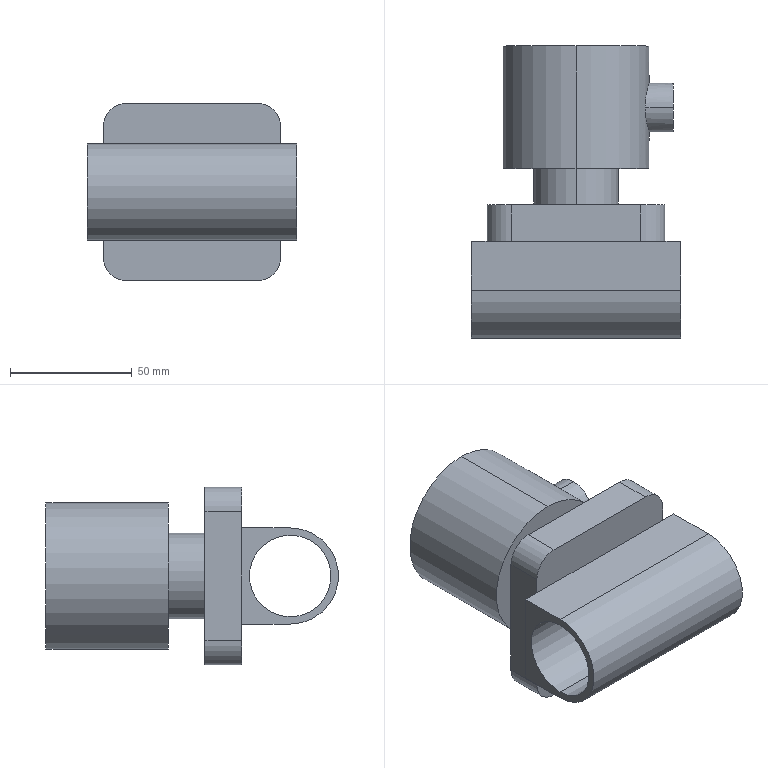Part | SolidWorks | features ICE 5, ExtruThin 1 | 1 solid | 29 faces | box 86 x 120 x 73 mm | volume 283263 mm3 | plane 16 | cylinder 13 | commonest cylinder face diameters 20 x6 33.5 x2 35 x2 60 x2 39.5 x1
STEP:
#1=CARTESIAN_POINT('',(28.284,75.,-10.));
#2=VERTEX_POINT('',#1);
#3=CARTESIAN_POINT('',(28.284,75.,10.));
#4=VERTEX_POINT('',#3);
#5=CARTESIAN_POINT('',(28.284,75.,-10.));
#6=CARTESIAN_POINT('',(28.284,75.666,-10.));
#7=CARTESIAN_POINT('',(28.308,76.32,-9.934));
#8=CARTESIAN_POINT('',(28.374,77.283,-9.741));
#9=CARTESIAN_POINT('',(28.402,77.601,-9.661));
#10=CARTESIAN_POINT('',(28.467,78.232,-9.469));
#11=CARTESIAN_POINT('',(28.504,78.544,-9.357));
#12=CARTESIAN_POINT('',(28.626,79.45,-8.979));
#13=CARTESIAN_POINT('',(28.722,80.023,-8.672));
#14=CARTESIAN_POINT('',(28.879,80.835,-8.128));
#15=CARTESIAN_POINT('',(28.933,81.099,-7.931));
#16=CARTESIAN_POINT('',(29.044,81.603,-7.517));
#17=CARTESIAN_POINT('',(29.1,81.844,-7.299));
#18=CARTESIAN_POINT('',(29.266,82.53,-6.612));
#19=CARTESIAN_POINT('',(29.376,82.942,-6.112));
#20=CARTESIAN_POINT('',(29.582,83.674,-5.02));
#21=CARTESIAN_POINT('',(29.675,83.981,-4.445));
#22=CARTESIAN_POINT('',(29.791,84.357,-3.544));
#23=CARTESIAN_POINT('',(29.827,84.467,-3.237));
#24=CARTESIAN_POINT('',(29.888,84.66,-2.608));
#25=CARTESIAN_POINT('',(29.915,84.741,-2.285));
#26=CARTESIAN_POINT('',(29.978,84.935,-1.315));
#27=CARTESIAN_POINT('',(30.,85.,-0.6623));
#28=CARTESIAN_POINT('',(30.,85.,0.3243));
#29=CARTESIAN_POINT('',(29.995,84.984,0.6555));
#30=CARTESIAN_POINT('',(29.973,84.918,1.317));
#31=CARTESIAN_POINT('',(29.957,84.87,1.643));
#32=CARTESIAN_POINT('',(29.893,84.676,2.608));
#33=CARTESIAN_POINT('',(29.831,84.486,3.234));
#34=CARTESIAN_POINT('',(29.714,84.106,4.147));
#35=CARTESIAN_POINT('',(29.67,83.964,4.445));
#36=CARTESIAN_POINT('',(29.579,83.655,5.02));
#37=CARTESIAN_POINT('',(29.53,83.487,5.298));
#38=CARTESIAN_POINT('',(29.428,83.126,5.837));
#39=CARTESIAN_POINT('',(29.375,82.932,6.098));
#40=CARTESIAN_POINT('',(29.266,82.518,6.602));
#41=CARTESIAN_POINT('',(29.209,82.297,6.846));
#42=CARTESIAN_POINT('',(29.042,81.606,7.536));
#43=CARTESIAN_POINT('',(28.931,81.106,7.946));
#44=CARTESIAN_POINT('',(28.722,80.026,8.67));
#45=CARTESIAN_POINT('',(28.625,79.441,8.984));
#46=CARTESIAN_POINT('',(28.463,78.237,9.484));
#47=CARTESIAN_POINT('',(28.397,77.613,9.675));
#48=CARTESIAN_POINT('',(28.33,76.643,9.87));
#49=CARTESIAN_POINT('',(28.313,76.312,9.919));
#50=CARTESIAN_POINT('',(28.29,75.656,9.984));
#51=CARTESIAN_POINT('',(28.284,75.328,10.));
#52=CARTESIAN_POINT('',(28.284,75.,10.));
#53=B_SPLINE_CURVE_WITH_KNOTS('',3,(#5,#6,#7,#8,#9,#10,#11,#12,#13,#14,#15,#16,#17,#18,#19,#20,#21,#22,#23,#24,#25,#26,#27,#28,#29,#30,#31,#32,#33,#34,#35,#36,#37,#38,#39,#40,#41,#42,#43,#44,#45,#46,#47,#48,#49,#50,#51,#52),.UNSPECIFIED.,.F.,.F.,(4,2,2,2,2,2,2,2,2,2,2,2,2,2,2,2,2,2,2,2,2,2,2,4),(0.,0.001968,0.002952,0.003936,0.005905,0.006889,0.007873,0.009841,0.01181,0.01279,0.01378,0.01575,0.01673,0.01771,0.01968,0.02067,0.02165,0.02263,0.02362,0.02559,0.02755,0.02952,0.03051,0.03149),.UNSPECIFIED.);
#54=EDGE_CURVE('',#2,#4,#53,.T.);
#55=ORIENTED_EDGE('',*,*,#54,.T.);
#56=CARTESIAN_POINT('',(40.,75.,10.));
#57=VERTEX_POINT('',#56);
#58=CARTESIAN_POINT('',(-43.001,75.,10.));
#59=DIRECTION('',(1.,0.,0.));
#60=VECTOR('',#59,1000.);
#61=LINE('',#58,#60);
#62=EDGE_CURVE('',#4,#57,#61,.T.);
#63=ORIENTED_EDGE('',*,*,#62,.T.);
#64=CARTESIAN_POINT('',(40.,75.,-10.));
#65=VERTEX_POINT('',#64);
#66=CARTESIAN_POINT('',(40.,75.,0.));
#67=DIRECTION('',(1.,0.,0.));
#68=DIRECTION('',(0.,0.,-1.));
#69=AXIS2_PLACEMENT_3D('',#66,#67,#68);
#70=CIRCLE('',#69,10.);
#71=EDGE_CURVE('',#65,#57,#70,.T.);
#72=ORIENTED_EDGE('',*,*,#71,.F.);
#73=CARTESIAN_POINT('',(-43.001,75.,-10.));
#74=DIRECTION('',(1.,0.,0.));
#75=VECTOR('',#74,1000.);
#76=LINE('',#73,#75);
#77=EDGE_CURVE('',#2,#65,#76,.T.);
#78=ORIENTED_EDGE('',*,*,#77,.F.);
#79=EDGE_LOOP('',(#55,#63,#72,#78));
#80=FACE_OUTER_BOUND('',#79,.T.);
#81=CARTESIAN_POINT('',(-43.001,75.,0.));
#82=DIRECTION('',(1.,0.,0.));
#83=DIRECTION('',(0.,0.,-1.));
#84=AXIS2_PLACEMENT_3D('',#81,#82,#83);
#85=CYLINDRICAL_SURFACE('',#84,10.);
#86=ADVANCED_FACE('',(#80),#85,.T.);
#87=ORIENTED_EDGE('',*,*,#54,.F.);
#88=CARTESIAN_POINT('',(28.284,75.,10.));
#89=CARTESIAN_POINT('',(28.284,74.672,10.));
#90=CARTESIAN_POINT('',(28.29,74.344,9.984));
#91=CARTESIAN_POINT('',(28.313,73.689,9.919));
#92=CARTESIAN_POINT('',(28.33,73.36,9.87));
#93=CARTESIAN_POINT('',(28.397,72.387,9.675));
#94=CARTESIAN_POINT('',(28.463,71.762,9.484));
#95=CARTESIAN_POINT('',(28.625,70.556,8.982));
#96=CARTESIAN_POINT('',(28.723,69.971,8.668));
#97=CARTESIAN_POINT('',(28.931,68.892,7.944));
#98=CARTESIAN_POINT('',(29.043,68.391,7.533));
#99=CARTESIAN_POINT('',(29.211,67.699,6.841));
#100=CARTESIAN_POINT('',(29.267,67.478,6.597));
#101=CARTESIAN_POINT('',(29.375,67.065,6.095));
#102=CARTESIAN_POINT('',(29.428,66.872,5.835));
#103=CARTESIAN_POINT('',(29.53,66.512,5.296));
#104=CARTESIAN_POINT('',(29.579,66.344,5.018));
#105=CARTESIAN_POINT('',(29.671,66.036,4.444));
#106=CARTESIAN_POINT('',(29.714,65.894,4.145));
#107=CARTESIAN_POINT('',(29.832,65.514,3.233));
#108=CARTESIAN_POINT('',(29.893,65.324,2.609));
#109=CARTESIAN_POINT('',(29.957,65.131,1.646));
#110=CARTESIAN_POINT('',(29.973,65.082,1.32));
#111=CARTESIAN_POINT('',(29.995,65.016,0.6609));
#112=CARTESIAN_POINT('',(30.,65.,0.328));
#113=CARTESIAN_POINT('',(30.,65.,-0.6604));
#114=CARTESIAN_POINT('',(29.978,65.065,-1.313));
#115=CARTESIAN_POINT('',(29.915,65.258,-2.282));
#116=CARTESIAN_POINT('',(29.888,65.34,-2.606));
#117=CARTESIAN_POINT('',(29.827,65.532,-3.235));
#118=CARTESIAN_POINT('',(29.792,65.643,-3.543));
#119=CARTESIAN_POINT('',(29.714,65.894,-4.145));
#120=CARTESIAN_POINT('',(29.671,66.034,-4.44));
#121=CARTESIAN_POINT('',(29.579,66.342,-5.015));
#122=CARTESIAN_POINT('',(29.53,66.512,-5.297));
#123=CARTESIAN_POINT('',(29.376,67.059,-6.113));
#124=CARTESIAN_POINT('',(29.266,67.471,-6.614));
#125=CARTESIAN_POINT('',(29.099,68.159,-7.301));
#126=CARTESIAN_POINT('',(29.043,68.4,-7.519));
#127=CARTESIAN_POINT('',(28.932,68.905,-7.935));
#128=CARTESIAN_POINT('',(28.878,69.169,-8.13));
#129=CARTESIAN_POINT('',(28.722,69.979,-8.672));
#130=CARTESIAN_POINT('',(28.626,70.55,-8.979));
#131=CARTESIAN_POINT('',(28.504,71.457,-9.357));
#132=CARTESIAN_POINT('',(28.467,71.769,-9.469));
#133=CARTESIAN_POINT('',(28.402,72.399,-9.661));
#134=CARTESIAN_POINT('',(28.374,72.717,-9.741));
#135=CARTESIAN_POINT('',(28.308,73.68,-9.934));
#136=CARTESIAN_POINT('',(28.284,74.334,-10.));
#137=CARTESIAN_POINT('',(28.284,75.,-10.));
#138=B_SPLINE_CURVE_WITH_KNOTS('',3,(#88,#89,#90,#91,#92,#93,#94,#95,#96,#97,#98,#99,#100,#101,#102,#103,#104,#105,#106,#107,#108,#109,#110,#111,#112,#113,#114,#115,#116,#117,#118,#119,#120,#121,#122,#123,#124,#125,#126,#127,#128,#129,#130,#131,#132,#133,#134,#135,#136,#137),.UNSPECIFIED.,.F.,.F.,(4,2,2,2,2,2,2,2,2,2,2,2,2,2,2,2,2,2,2,2,2,2,2,2,4),(0.03149,0.03247,0.03346,0.03543,0.03739,0.03936,0.04035,0.04133,0.04231,0.0433,0.04526,0.04625,0.04723,0.0492,0.05018,0.05117,0.05215,0.05313,0.0551,0.05609,0.05707,0.05904,0.06002,0.06101,0.06297),.UNSPECIFIED.);
#139=EDGE_CURVE('',#4,#2,#138,.T.);
#140=ORIENTED_EDGE('',*,*,#139,.F.);
#141=EDGE_LOOP('',(#87,#140));
#142=FACE_BOUND('',#141,.T.);
#143=CARTESIAN_POINT('',(0.,100.25,30.));
#144=VERTEX_POINT('',#143);
#145=CARTESIAN_POINT('',(0.,100.25,-30.));
#146=VERTEX_POINT('',#145);
#147=CARTESIAN_POINT('',(0.,100.25,0.));
#148=DIRECTION('',(0.,1.,0.));
#149=DIRECTION('',(0.,0.,1.));
#150=AXIS2_PLACEMENT_3D('',#147,#148,#149);
#151=CIRCLE('',#150,30.);
#152=EDGE_CURVE('',#144,#146,#151,.T.);
#153=ORIENTED_EDGE('',*,*,#152,.F.);
#154=CARTESIAN_POINT('',(0.,50.,30.));
#155=VERTEX_POINT('',#154);
#156=CARTESIAN_POINT('',(0.,100.25,30.));
#157=DIRECTION('',(0.,-1.,0.));
#158=VECTOR('',#157,1000.);
#159=LINE('',#156,#158);
#160=EDGE_CURVE('',#144,#155,#159,.T.);
#161=ORIENTED_EDGE('',*,*,#160,.T.);
#162=CARTESIAN_POINT('',(0.,50.,-30.));
#163=VERTEX_POINT('',#162);
#164=CARTESIAN_POINT('',(0.,50.,0.));
#165=DIRECTION('',(0.,1.,0.));
#166=DIRECTION('',(0.,0.,1.));
#167=AXIS2_PLACEMENT_3D('',#164,#165,#166);
#168=CIRCLE('',#167,30.);
#169=EDGE_CURVE('',#155,#163,#168,.T.);
#170=ORIENTED_EDGE('',*,*,#169,.T.);
#171=CARTESIAN_POINT('',(0.,100.25,-30.));
#172=DIRECTION('',(0.,-1.,0.));
#173=VECTOR('',#172,1000.);
#174=LINE('',#171,#173);
#175=EDGE_CURVE('',#146,#163,#174,.T.);
#176=ORIENTED_EDGE('',*,*,#175,.F.);
#177=EDGE_LOOP('',(#153,#161,#170,#176));
#178=FACE_OUTER_BOUND('',#177,.T.);
#179=CARTESIAN_POINT('',(0.,100.25,0.));
#180=DIRECTION('',(0.,-1.,0.));
#181=DIRECTION('',(0.,0.,-1.));
#182=AXIS2_PLACEMENT_3D('',#179,#180,#181);
#183=CYLINDRICAL_SURFACE('',#182,30.);
#184=ADVANCED_FACE('',(#142,#178),#183,.T.);
#185=CARTESIAN_POINT('',(0.,50.,17.5));
#186=VERTEX_POINT('',#185);
#187=CARTESIAN_POINT('',(0.,50.,-17.5));
#188=VERTEX_POINT('',#187);
#189=CARTESIAN_POINT('',(0.,50.,0.));
#190=DIRECTION('',(0.,1.,0.));
#191=DIRECTION('',(0.,0.,1.));
#192=AXIS2_PLACEMENT_3D('',#189,#190,#191);
#193=CIRCLE('',#192,17.5);
#194=EDGE_CURVE('',#186,#188,#193,.T.);
#195=ORIENTED_EDGE('',*,*,#194,.F.);
#196=CARTESIAN_POINT('',(0.,35.,17.5));
#197=VERTEX_POINT('',#196);
#198=CARTESIAN_POINT('',(0.,50.,17.5));
#199=DIRECTION('',(0.,-1.,0.));
#200=VECTOR('',#199,1000.);
#201=LINE('',#198,#200);
#202=EDGE_CURVE('',#186,#197,#201,.T.);
#203=ORIENTED_EDGE('',*,*,#202,.T.);
#204=CARTESIAN_POINT('',(0.,35.,-17.5));
#205=VERTEX_POINT('',#204);
#206=CARTESIAN_POINT('',(0.,35.,0.));
#207=DIRECTION('',(0.,1.,0.));
#208=DIRECTION('',(0.,0.,-1.));
#209=AXIS2_PLACEMENT_3D('',#206,#207,#208);
#210=CIRCLE('',#209,17.5);
#211=EDGE_CURVE('',#197,#205,#210,.T.);
#212=ORIENTED_EDGE('',*,*,#211,.T.);
#213=CARTESIAN_POINT('',(0.,50.,-17.5));
#214=DIRECTION('',(0.,-1.,0.));
#215=VECTOR('',#214,1000.);
#216=LINE('',#213,#215);
#217=EDGE_CURVE('',#188,#205,#216,.T.);
#218=ORIENTED_EDGE('',*,*,#217,.F.);
#219=EDGE_LOOP('',(#195,#203,#212,#218));
#220=FACE_OUTER_BOUND('',#219,.T.);
#221=CARTESIAN_POINT('',(0.,50.,0.));
#222=DIRECTION('',(0.,-1.,0.));
#223=DIRECTION('',(0.,0.,-1.));
#224=AXIS2_PLACEMENT_3D('',#221,#222,#223);
#225=CYLINDRICAL_SURFACE('',#224,17.5);
#226=ADVANCED_FACE('',(#220),#225,.T.);
#227=CARTESIAN_POINT('',(43.,0.,16.75));
#228=VERTEX_POINT('',#227);
#229=CARTESIAN_POINT('',(43.,0.,-16.75));
#230=VERTEX_POINT('',#229);
#231=CARTESIAN_POINT('',(43.,0.,0.));
#232=DIRECTION('',(1.,0.,0.));
#233=DIRECTION('',(0.,0.,-1.));
#234=AXIS2_PLACEMENT_3D('',#231,#232,#233);
#235=CIRCLE('',#234,16.75);
#236=EDGE_CURVE('',#228,#230,#235,.T.);
#237=ORIENTED_EDGE('',*,*,#236,.T.);
#238=CARTESIAN_POINT('',(-43.,0.,-16.75));
#239=VERTEX_POINT('',#238);
#240=CARTESIAN_POINT('',(43.,0.,-16.75));
#241=DIRECTION('',(-1.,0.,0.));
#242=VECTOR('',#241,1000.);
#243=LINE('',#240,#242);
#244=EDGE_CURVE('',#230,#239,#243,.T.);
#245=ORIENTED_EDGE('',*,*,#244,.T.);
#246=CARTESIAN_POINT('',(-43.,0.,16.75));
#247=VERTEX_POINT('',#246);
#248=CARTESIAN_POINT('',(-43.,0.,0.));
#249=DIRECTION('',(1.,0.,0.));
#250=DIRECTION('',(0.,0.,-1.));
#251=AXIS2_PLACEMENT_3D('',#248,#249,#250);
#252=CIRCLE('',#251,16.75);
#253=EDGE_CURVE('',#247,#239,#252,.T.);
#254=ORIENTED_EDGE('',*,*,#253,.F.);
#255=CARTESIAN_POINT('',(43.,0.,16.75));
#256=DIRECTION('',(-1.,0.,0.));
#257=VECTOR('',#256,1000.);
#258=LINE('',#255,#257);
#259=EDGE_CURVE('',#228,#247,#258,.T.);
#260=ORIENTED_EDGE('',*,*,#259,.F.);
#261=EDGE_LOOP('',(#237,#245,#254,#260));
#262=FACE_OUTER_BOUND('',#261,.T.);
#263=CARTESIAN_POINT('',(43.,0.,0.));
#264=DIRECTION('',(-1.,0.,0.));
#265=DIRECTION('',(0.,0.,1.));
#266=AXIS2_PLACEMENT_3D('',#263,#264,#265);
#267=CYLINDRICAL_SURFACE('',#266,16.75);
#268=ADVANCED_FACE('',(#262),#267,.F.);
#269=CARTESIAN_POINT('',(-36.5,20.,-19.75));
#270=VERTEX_POINT('',#269);
#271=CARTESIAN_POINT('',(-36.5,20.,19.75));
#272=VERTEX_POINT('',#271);
#273=CARTESIAN_POINT('',(-36.5,20.,-26.5));
#274=DIRECTION('',(0.,0.,1.));
#275=VECTOR('',#274,1000.);
#276=LINE('',#273,#275);
#277=EDGE_CURVE('',#270,#272,#276,.T.);
#278=ORIENTED_EDGE('',*,*,#277,.F.);
#279=CARTESIAN_POINT('',(-43.,20.,-19.75));
#280=VERTEX_POINT('',#279);
#281=CARTESIAN_POINT('',(-87.275,20.,-19.75));
#282=DIRECTION('',(1.,0.,0.));
#283=VECTOR('',#282,1000.);
#284=LINE('',#281,#283);
#285=EDGE_CURVE('',#280,#270,#284,.T.);
#286=ORIENTED_EDGE('',*,*,#285,.F.);
#287=CARTESIAN_POINT('',(-43.,20.,19.75));
#288=VERTEX_POINT('',#287);
#289=CARTESIAN_POINT('',(-43.,20.,19.75));
#290=DIRECTION('',(0.,0.,-1.));
#291=VECTOR('',#290,1000.);
#292=LINE('',#289,#291);
#293=EDGE_CURVE('',#288,#280,#292,.T.);
#294=ORIENTED_EDGE('',*,*,#293,.F.);
#295=CARTESIAN_POINT('',(-87.275,20.,19.75));
#296=DIRECTION('',(1.,0.,0.));
#297=VECTOR('',#296,1000.);
#298=LINE('',#295,#297);
#299=EDGE_CURVE('',#288,#272,#298,.T.);
#300=ORIENTED_EDGE('',*,*,#299,.T.);
#301=EDGE_LOOP('',(#278,#286,#294,#300));
#302=FACE_OUTER_BOUND('',#301,.T.);
#303=CARTESIAN_POINT('',(-87.275,20.,19.75));
#304=DIRECTION('',(0.,1.,0.));
#305=DIRECTION('',(0.,0.,1.));
#306=AXIS2_PLACEMENT_3D('',#303,#304,#305);
#307=PLANE('',#306);
#308=ADVANCED_FACE('',(#302),#307,.T.);
#309=CARTESIAN_POINT('',(43.,0.,19.75));
#310=VERTEX_POINT('',#309);
#311=CARTESIAN_POINT('',(43.,0.,-19.75));
#312=VERTEX_POINT('',#311);
#313=CARTESIAN_POINT('',(43.,0.,0.));
#314=DIRECTION('',(1.,0.,0.));
#315=DIRECTION('',(0.,0.,-1.));
#316=AXIS2_PLACEMENT_3D('',#313,#314,#315);
#317=CIRCLE('',#316,19.75);
#318=EDGE_CURVE('',#310,#312,#317,.T.);
#319=ORIENTED_EDGE('',*,*,#318,.T.);
#320=CARTESIAN_POINT('',(43.,20.,-19.75));
#321=VERTEX_POINT('',#320);
#322=CARTESIAN_POINT('',(43.,0.,-19.75));
#323=DIRECTION('',(0.,1.,0.));
#324=VECTOR('',#323,1000.);
#325=LINE('',#322,#324);
#326=EDGE_CURVE('',#312,#321,#325,.T.);
#327=ORIENTED_EDGE('',*,*,#326,.T.);
#328=CARTESIAN_POINT('',(43.,20.,19.75));
#329=VERTEX_POINT('',#328);
#330=CARTESIAN_POINT('',(43.,20.,19.75));
#331=DIRECTION('',(0.,0.,1.));
#332=VECTOR('',#331,1000.);
#333=LINE('',#330,#332);
#334=EDGE_CURVE('',#321,#329,#333,.T.);
#335=ORIENTED_EDGE('',*,*,#334,.T.);
#336=CARTESIAN_POINT('',(43.,0.,19.75));
#337=DIRECTION('',(0.,-1.,0.));
#338=VECTOR('',#337,1000.);
#339=LINE('',#336,#338);
#340=EDGE_CURVE('',#329,#310,#339,.T.);
#341=ORIENTED_EDGE('',*,*,#340,.T.);
#342=EDGE_LOOP('',(#319,#327,#335,#341));
#343=FACE_OUTER_BOUND('',#342,.T.);
#344=ORIENTED_EDGE('',*,*,#236,.F.);
#345=CARTESIAN_POINT('',(43.,0.,0.));
#346=DIRECTION('',(1.,0.,0.));
#347=DIRECTION('',(0.,0.,-1.));
#348=AXIS2_PLACEMENT_3D('',#345,#346,#347);
#349=CIRCLE('',#348,16.75);
#350=EDGE_CURVE('',#230,#228,#349,.T.);
#351=ORIENTED_EDGE('',*,*,#350,.F.);
#352=EDGE_LOOP('',(#344,#351));
#353=FACE_BOUND('',#352,.T.);
#354=CARTESIAN_POINT('',(43.,0.,0.));
#355=DIRECTION('',(1.,0.,0.));
#356=DIRECTION('',(0.,0.,-1.));
#357=AXIS2_PLACEMENT_3D('',#354,#355,#356);
#358=PLANE('',#357);
#359=ADVANCED_FACE('',(#343,#353),#358,.T.);
#360=CARTESIAN_POINT('',(-43.,0.,19.75));
#361=VERTEX_POINT('',#360);
#362=CARTESIAN_POINT('',(-43.,0.,-19.75));
#363=VERTEX_POINT('',#362);
#364=CARTESIAN_POINT('',(-43.,0.,0.));
#365=DIRECTION('',(1.,0.,0.));
#366=DIRECTION('',(0.,0.,-1.));
#367=AXIS2_PLACEMENT_3D('',#364,#365,#366);
#368=CIRCLE('',#367,19.75);
#369=EDGE_CURVE('',#361,#363,#368,.T.);
#370=ORIENTED_EDGE('',*,*,#369,.F.);
#371=CARTESIAN_POINT('',(-43.,0.,19.75));
#372=DIRECTION('',(0.,1.,0.));
#373=VECTOR('',#372,1000.);
#374=LINE('',#371,#373);
#375=EDGE_CURVE('',#361,#288,#374,.T.);
#376=ORIENTED_EDGE('',*,*,#375,.T.);
#377=ORIENTED_EDGE('',*,*,#293,.T.);
#378=CARTESIAN_POINT('',(-43.,0.,-19.75));
#379=DIRECTION('',(0.,-1.,0.));
#380=VECTOR('',#379,1000.);
#381=LINE('',#378,#380);
#382=EDGE_CURVE('',#280,#363,#381,.T.);
#383=ORIENTED_EDGE('',*,*,#382,.T.);
#384=EDGE_LOOP('',(#370,#376,#377,#383));
#385=FACE_OUTER_BOUND('',#384,.T.);
#386=ORIENTED_EDGE('',*,*,#253,.T.);
#387=CARTESIAN_POINT('',(-43.,0.,0.));
#388=DIRECTION('',(1.,0.,0.));
#389=DIRECTION('',(0.,0.,-1.));
#390=AXIS2_PLACEMENT_3D('',#387,#388,#389);
#391=CIRCLE('',#390,16.75);
#392=EDGE_CURVE('',#239,#247,#391,.T.);
#393=ORIENTED_EDGE('',*,*,#392,.T.);
#394=EDGE_LOOP('',(#386,#393));
#395=FACE_BOUND('',#394,.T.);
#396=CARTESIAN_POINT('',(-43.,0.,0.));
#397=DIRECTION('',(1.,0.,0.));
#398=DIRECTION('',(0.,0.,-1.));
#399=AXIS2_PLACEMENT_3D('',#396,#397,#398);
#400=PLANE('',#399);
#401=ADVANCED_FACE('',(#385,#395),#400,.F.);
#402=ORIENTED_EDGE('',*,*,#318,.F.);
#403=CARTESIAN_POINT('',(-87.275,0.,19.75));
#404=DIRECTION('',(1.,0.,0.));
#405=VECTOR('',#404,1000.);
#406=LINE('',#403,#405);
#407=EDGE_CURVE('',#361,#310,#406,.T.);
#408=ORIENTED_EDGE('',*,*,#407,.F.);
#409=ORIENTED_EDGE('',*,*,#369,.T.);
#410=CARTESIAN_POINT('',(-87.275,0.,-19.75));
#411=DIRECTION('',(1.,0.,0.));
#412=VECTOR('',#411,1000.);
#413=LINE('',#410,#412);
#414=EDGE_CURVE('',#363,#312,#413,.T.);
#415=ORIENTED_EDGE('',*,*,#414,.T.);
#416=EDGE_LOOP('',(#402,#408,#409,#415));
#417=FACE_OUTER_BOUND('',#416,.T.);
#418=CARTESIAN_POINT('',(43.,0.,0.));
#419=DIRECTION('',(-1.,0.,0.));
#420=DIRECTION('',(0.,0.,1.));
#421=AXIS2_PLACEMENT_3D('',#418,#419,#420);
#422=CYLINDRICAL_SURFACE('',#421,19.75);
#423=ADVANCED_FACE('',(#417),#422,.T.);
#424=ORIENTED_EDGE('',*,*,#244,.F.);
#425=ORIENTED_EDGE('',*,*,#350,.T.);
#426=ORIENTED_EDGE('',*,*,#259,.T.);
#427=ORIENTED_EDGE('',*,*,#392,.F.);
#428=EDGE_LOOP('',(#424,#425,#426,#427));
#429=FACE_OUTER_BOUND('',#428,.T.);
#430=CARTESIAN_POINT('',(43.,0.,0.));
#431=DIRECTION('',(-1.,0.,0.));
#432=DIRECTION('',(0.,0.,1.));
#433=AXIS2_PLACEMENT_3D('',#430,#431,#432);
#434=CYLINDRICAL_SURFACE('',#433,16.75);
#435=ADVANCED_FACE('',(#429),#434,.F.);
#436=ORIENTED_EDGE('',*,*,#375,.F.);
#437=ORIENTED_EDGE('',*,*,#407,.T.);
#438=ORIENTED_EDGE('',*,*,#340,.F.);
#439=CARTESIAN_POINT('',(36.5,20.,19.75));
#440=VERTEX_POINT('',#439);
#441=CARTESIAN_POINT('',(-87.275,20.,19.75));
#442=DIRECTION('',(1.,0.,0.));
#443=VECTOR('',#442,1000.);
#444=LINE('',#441,#443);
#445=EDGE_CURVE('',#440,#329,#444,.T.);
#446=ORIENTED_EDGE('',*,*,#445,.F.);
#447=CARTESIAN_POINT('',(-87.275,20.,19.75));
#448=DIRECTION('',(1.,0.,0.));
#449=VECTOR('',#448,1000.);
#450=LINE('',#447,#449);
#451=EDGE_CURVE('',#272,#440,#450,.T.);
#452=ORIENTED_EDGE('',*,*,#451,.F.);
#453=ORIENTED_EDGE('',*,*,#299,.F.);
#454=EDGE_LOOP('',(#436,#437,#438,#446,#452,#453));
#455=FACE_OUTER_BOUND('',#454,.T.);
#456=CARTESIAN_POINT('',(-87.275,0.,19.75));
#457=DIRECTION('',(0.,0.,1.));
#458=DIRECTION('',(1.,0.,0.));
#459=AXIS2_PLACEMENT_3D('',#456,#457,#458);
#460=PLANE('',#459);
#461=ADVANCED_FACE('',(#455),#460,.T.);
#462=CARTESIAN_POINT('',(36.5,20.,-19.75));
#463=VERTEX_POINT('',#462);
#464=CARTESIAN_POINT('',(36.5,20.,-26.5));
#465=DIRECTION('',(0.,0.,-1.));
#466=VECTOR('',#465,1000.);
#467=LINE('',#464,#466);
#468=EDGE_CURVE('',#440,#463,#467,.T.);
#469=ORIENTED_EDGE('',*,*,#468,.F.);
#470=ORIENTED_EDGE('',*,*,#445,.T.);
#471=ORIENTED_EDGE('',*,*,#334,.F.);
#472=CARTESIAN_POINT('',(-87.275,20.,-19.75));
#473=DIRECTION('',(1.,0.,0.));
#474=VECTOR('',#473,1000.);
#475=LINE('',#472,#474);
#476=EDGE_CURVE('',#463,#321,#475,.T.);
#477=ORIENTED_EDGE('',*,*,#476,.F.);
#478=EDGE_LOOP('',(#469,#470,#471,#477));
#479=FACE_OUTER_BOUND('',#478,.T.);
#480=CARTESIAN_POINT('',(-87.275,20.,19.75));
#481=DIRECTION('',(0.,1.,0.));
#482=DIRECTION('',(0.,0.,1.));
#483=AXIS2_PLACEMENT_3D('',#480,#481,#482);
#484=PLANE('',#483);
#485=ADVANCED_FACE('',(#479),#484,.T.);
#486=ORIENTED_EDGE('',*,*,#382,.F.);
#487=ORIENTED_EDGE('',*,*,#285,.T.);
#488=CARTESIAN_POINT('',(-87.275,20.,-19.75));
#489=DIRECTION('',(1.,0.,0.));
#490=VECTOR('',#489,1000.);
#491=LINE('',#488,#490);
#492=EDGE_CURVE('',#270,#463,#491,.T.);
#493=ORIENTED_EDGE('',*,*,#492,.T.);
#494=ORIENTED_EDGE('',*,*,#476,.T.);
#495=ORIENTED_EDGE('',*,*,#326,.F.);
#496=ORIENTED_EDGE('',*,*,#414,.F.);
#497=EDGE_LOOP('',(#486,#487,#493,#494,#495,#496));
#498=FACE_OUTER_BOUND('',#497,.T.);
#499=CARTESIAN_POINT('',(-87.275,0.,-19.75));
#500=DIRECTION('',(0.,0.,-1.));
#501=DIRECTION('',(-1.,0.,0.));
#502=AXIS2_PLACEMENT_3D('',#499,#500,#501);
#503=PLANE('',#502);
#504=ADVANCED_FACE('',(#498),#503,.T.);
#505=ORIENTED_EDGE('',*,*,#492,.F.);
#506=CARTESIAN_POINT('',(-36.5,20.,-26.5));
#507=VERTEX_POINT('',#506);
#508=CARTESIAN_POINT('',(-36.5,20.,-26.5));
#509=DIRECTION('',(0.,0.,1.));
#510=VECTOR('',#509,1000.);
#511=LINE('',#508,#510);
#512=EDGE_CURVE('',#507,#270,#511,.T.);
#513=ORIENTED_EDGE('',*,*,#512,.F.);
#514=CARTESIAN_POINT('',(-26.5,20.,-36.5));
#515=VERTEX_POINT('',#514);
#516=CARTESIAN_POINT('',(-26.5,20.,-26.5));
#517=DIRECTION('',(0.,1.,0.));
#518=DIRECTION('',(0.,0.,1.));
#519=AXIS2_PLACEMENT_3D('',#516,#517,#518);
#520=CIRCLE('',#519,10.);
#521=EDGE_CURVE('',#515,#507,#520,.T.);
#522=ORIENTED_EDGE('',*,*,#521,.F.);
#523=CARTESIAN_POINT('',(26.5,20.,-36.5));
#524=VERTEX_POINT('',#523);
#525=CARTESIAN_POINT('',(-26.5,20.,-36.5));
#526=DIRECTION('',(-1.,0.,0.));
#527=VECTOR('',#526,1000.);
#528=LINE('',#525,#527);
#529=EDGE_CURVE('',#524,#515,#528,.T.);
#530=ORIENTED_EDGE('',*,*,#529,.F.);
#531=CARTESIAN_POINT('',(36.5,20.,-26.5));
#532=VERTEX_POINT('',#531);
#533=CARTESIAN_POINT('',(26.5,20.,-26.5));
#534=DIRECTION('',(0.,1.,0.));
#535=DIRECTION('',(0.,0.,1.));
#536=AXIS2_PLACEMENT_3D('',#533,#534,#535);
#537=CIRCLE('',#536,10.);
#538=EDGE_CURVE('',#532,#524,#537,.T.);
#539=ORIENTED_EDGE('',*,*,#538,.F.);
#540=CARTESIAN_POINT('',(36.5,20.,-26.5));
#541=DIRECTION('',(0.,0.,-1.));
#542=VECTOR('',#541,1000.);
#543=LINE('',#540,#542);
#544=EDGE_CURVE('',#463,#532,#543,.T.);
#545=ORIENTED_EDGE('',*,*,#544,.F.);
#546=EDGE_LOOP('',(#505,#513,#522,#530,#539,#545));
#547=FACE_OUTER_BOUND('',#546,.T.);
#548=CARTESIAN_POINT('',(-26.5,20.,26.5));
#549=DIRECTION('',(0.,-1.,0.));
#550=DIRECTION('',(0.,0.,-1.));
#551=AXIS2_PLACEMENT_3D('',#548,#549,#550);
#552=PLANE('',#551);
#553=ADVANCED_FACE('',(#547),#552,.T.);
#554=CARTESIAN_POINT('',(-36.5,35.,26.5));
#555=VERTEX_POINT('',#554);
#556=CARTESIAN_POINT('',(-26.5,35.,36.5));
#557=VERTEX_POINT('',#556);
#558=CARTESIAN_POINT('',(-26.5,35.,26.5));
#559=DIRECTION('',(0.,1.,0.));
#560=DIRECTION('',(0.,0.,-1.));
#561=AXIS2_PLACEMENT_3D('',#558,#559,#560);
#562=CIRCLE('',#561,10.);
#563=EDGE_CURVE('',#555,#557,#562,.T.);
#564=ORIENTED_EDGE('',*,*,#563,.T.);
#565=CARTESIAN_POINT('',(26.5,35.,36.5));
#566=VERTEX_POINT('',#565);
#567=CARTESIAN_POINT('',(-26.5,35.,36.5));
#568=DIRECTION('',(1.,0.,0.));
#569=VECTOR('',#568,1000.);
#570=LINE('',#567,#569);
#571=EDGE_CURVE('',#557,#566,#570,.T.);
#572=ORIENTED_EDGE('',*,*,#571,.T.);
#573=CARTESIAN_POINT('',(36.5,35.,26.5));
#574=VERTEX_POINT('',#573);
#575=CARTESIAN_POINT('',(26.5,35.,26.5));
#576=DIRECTION('',(0.,1.,0.));
#577=DIRECTION('',(0.,0.,-1.));
#578=AXIS2_PLACEMENT_3D('',#575,#576,#577);
#579=CIRCLE('',#578,10.);
#580=EDGE_CURVE('',#566,#574,#579,.T.);
#581=ORIENTED_EDGE('',*,*,#580,.T.);
#582=CARTESIAN_POINT('',(36.5,35.,-26.5));
#583=VERTEX_POINT('',#582);
#584=CARTESIAN_POINT('',(36.5,35.,-26.5));
#585=DIRECTION('',(0.,0.,-1.));
#586=VECTOR('',#585,1000.);
#587=LINE('',#584,#586);
#588=EDGE_CURVE('',#574,#583,#587,.T.);
#589=ORIENTED_EDGE('',*,*,#588,.T.);
#590=CARTESIAN_POINT('',(26.5,35.,-36.5));
#591=VERTEX_POINT('',#590);
#592=CARTESIAN_POINT('',(26.5,35.,-26.5));
#593=DIRECTION('',(0.,1.,0.));
#594=DIRECTION('',(0.,0.,1.));
#595=AXIS2_PLACEMENT_3D('',#592,#593,#594);
#596=CIRCLE('',#595,10.);
#597=EDGE_CURVE('',#583,#591,#596,.T.);
#598=ORIENTED_EDGE('',*,*,#597,.T.);
#599=CARTESIAN_POINT('',(-26.5,35.,-36.5));
#600=VERTEX_POINT('',#599);
#601=CARTESIAN_POINT('',(-26.5,35.,-36.5));
#602=DIRECTION('',(-1.,0.,0.));
#603=VECTOR('',#602,1000.);
#604=LINE('',#601,#603);
#605=EDGE_CURVE('',#591,#600,#604,.T.);
#606=ORIENTED_EDGE('',*,*,#605,.T.);
#607=CARTESIAN_POINT('',(-36.5,35.,-26.5));
#608=VERTEX_POINT('',#607);
#609=CARTESIAN_POINT('',(-26.5,35.,-26.5));
#610=DIRECTION('',(0.,1.,0.));
#611=DIRECTION('',(0.,0.,1.));
#612=AXIS2_PLACEMENT_3D('',#609,#610,#611);
#613=CIRCLE('',#612,10.);
#614=EDGE_CURVE('',#600,#608,#613,.T.);
#615=ORIENTED_EDGE('',*,*,#614,.T.);
#616=CARTESIAN_POINT('',(-36.5,35.,-26.5));
#617=DIRECTION('',(0.,0.,1.));
#618=VECTOR('',#617,1000.);
#619=LINE('',#616,#618);
#620=EDGE_CURVE('',#608,#555,#619,.T.);
#621=ORIENTED_EDGE('',*,*,#620,.T.);
#622=EDGE_LOOP('',(#564,#572,#581,#589,#598,#606,#615,#621));
#623=FACE_OUTER_BOUND('',#622,.T.);
#624=CARTESIAN_POINT('',(0.,35.,0.));
#625=DIRECTION('',(0.,1.,0.));
#626=DIRECTION('',(0.,0.,-1.));
#627=AXIS2_PLACEMENT_3D('',#624,#625,#626);
#628=CIRCLE('',#627,17.5);
#629=EDGE_CURVE('',#205,#197,#628,.T.);
#630=ORIENTED_EDGE('',*,*,#629,.F.);
#631=ORIENTED_EDGE('',*,*,#211,.F.);
#632=EDGE_LOOP('',(#630,#631));
#633=FACE_BOUND('',#632,.T.);
#634=CARTESIAN_POINT('',(-26.5,35.,26.5));
#635=DIRECTION('',(0.,-1.,0.));
#636=DIRECTION('',(0.,0.,-1.));
#637=AXIS2_PLACEMENT_3D('',#634,#635,#636);
#638=PLANE('',#637);
#639=ADVANCED_FACE('',(#623,#633),#638,.F.);
#640=CARTESIAN_POINT('',(-36.5,20.,26.5));
#641=VERTEX_POINT('',#640);
#642=CARTESIAN_POINT('',(-26.5,20.,36.5));
#643=VERTEX_POINT('',#642);
#644=CARTESIAN_POINT('',(-26.5,20.,26.5));
#645=DIRECTION('',(0.,1.,0.));
#646=DIRECTION('',(0.,0.,-1.));
#647=AXIS2_PLACEMENT_3D('',#644,#645,#646);
#648=CIRCLE('',#647,10.);
#649=EDGE_CURVE('',#641,#643,#648,.T.);
#650=ORIENTED_EDGE('',*,*,#649,.T.);
#651=CARTESIAN_POINT('',(-26.5,35.,36.5));
#652=DIRECTION('',(0.,-1.,0.));
#653=VECTOR('',#652,1000.);
#654=LINE('',#651,#653);
#655=EDGE_CURVE('',#557,#643,#654,.T.);
#656=ORIENTED_EDGE('',*,*,#655,.F.);
#657=ORIENTED_EDGE('',*,*,#563,.F.);
#658=CARTESIAN_POINT('',(-36.5,35.,26.5));
#659=DIRECTION('',(0.,-1.,0.));
#660=VECTOR('',#659,1000.);
#661=LINE('',#658,#660);
#662=EDGE_CURVE('',#555,#641,#661,.T.);
#663=ORIENTED_EDGE('',*,*,#662,.T.);
#664=EDGE_LOOP('',(#650,#656,#657,#663));
#665=FACE_OUTER_BOUND('',#664,.T.);
#666=CARTESIAN_POINT('',(-26.5,35.,26.5));
#667=DIRECTION('',(0.,-1.,0.));
#668=DIRECTION('',(0.,0.,-1.));
#669=AXIS2_PLACEMENT_3D('',#666,#667,#668);
#670=CYLINDRICAL_SURFACE('',#669,10.);
#671=ADVANCED_FACE('',(#665),#670,.T.);
#672=CARTESIAN_POINT('',(26.5,20.,36.5));
#673=VERTEX_POINT('',#672);
#674=CARTESIAN_POINT('',(-26.5,20.,36.5));
#675=DIRECTION('',(1.,0.,0.));
#676=VECTOR('',#675,1000.);
#677=LINE('',#674,#676);
#678=EDGE_CURVE('',#643,#673,#677,.T.);
#679=ORIENTED_EDGE('',*,*,#678,.T.);
#680=CARTESIAN_POINT('',(26.5,35.,36.5));
#681=DIRECTION('',(0.,-1.,0.));
#682=VECTOR('',#681,1000.);
#683=LINE('',#680,#682);
#684=EDGE_CURVE('',#566,#673,#683,.T.);
#685=ORIENTED_EDGE('',*,*,#684,.F.);
#686=ORIENTED_EDGE('',*,*,#571,.F.);
#687=ORIENTED_EDGE('',*,*,#655,.T.);
#688=EDGE_LOOP('',(#679,#685,#686,#687));
#689=FACE_OUTER_BOUND('',#688,.T.);
#690=CARTESIAN_POINT('',(-26.5,35.,36.5));
#691=DIRECTION('',(0.,0.,-1.));
#692=DIRECTION('',(-1.,0.,0.));
#693=AXIS2_PLACEMENT_3D('',#690,#691,#692);
#694=PLANE('',#693);
#695=ADVANCED_FACE('',(#689),#694,.F.);
#696=CARTESIAN_POINT('',(36.5,20.,26.5));
#697=VERTEX_POINT('',#696);
#698=CARTESIAN_POINT('',(26.5,20.,26.5));
#699=DIRECTION('',(0.,1.,0.));
#700=DIRECTION('',(0.,0.,-1.));
#701=AXIS2_PLACEMENT_3D('',#698,#699,#700);
#702=CIRCLE('',#701,10.);
#703=EDGE_CURVE('',#673,#697,#702,.T.);
#704=ORIENTED_EDGE('',*,*,#703,.T.);
#705=CARTESIAN_POINT('',(36.5,35.,26.5));
#706=DIRECTION('',(0.,-1.,0.));
#707=VECTOR('',#706,1000.);
#708=LINE('',#705,#707);
#709=EDGE_CURVE('',#574,#697,#708,.T.);
#710=ORIENTED_EDGE('',*,*,#709,.F.);
#711=ORIENTED_EDGE('',*,*,#580,.F.);
#712=ORIENTED_EDGE('',*,*,#684,.T.);
#713=EDGE_LOOP('',(#704,#710,#711,#712));
#714=FACE_OUTER_BOUND('',#713,.T.);
#715=CARTESIAN_POINT('',(26.5,35.,26.5));
#716=DIRECTION('',(0.,-1.,0.));
#717=DIRECTION('',(0.,0.,-1.));
#718=AXIS2_PLACEMENT_3D('',#715,#716,#717);
#719=CYLINDRICAL_SURFACE('',#718,10.);
#720=ADVANCED_FACE('',(#714),#719,.T.);
#721=CARTESIAN_POINT('',(36.5,20.,-26.5));
#722=DIRECTION('',(0.,0.,-1.));
#723=VECTOR('',#722,1000.);
#724=LINE('',#721,#723);
#725=EDGE_CURVE('',#697,#440,#724,.T.);
#726=ORIENTED_EDGE('',*,*,#725,.T.);
#727=ORIENTED_EDGE('',*,*,#468,.T.);
#728=ORIENTED_EDGE('',*,*,#544,.T.);
#729=CARTESIAN_POINT('',(36.5,35.,-26.5));
#730=DIRECTION('',(0.,-1.,0.));
#731=VECTOR('',#730,1000.);
#732=LINE('',#729,#731);
#733=EDGE_CURVE('',#583,#532,#732,.T.);
#734=ORIENTED_EDGE('',*,*,#733,.F.);
#735=ORIENTED_EDGE('',*,*,#588,.F.);
#736=ORIENTED_EDGE('',*,*,#709,.T.);
#737=EDGE_LOOP('',(#726,#727,#728,#734,#735,#736));
#738=FACE_OUTER_BOUND('',#737,.T.);
#739=CARTESIAN_POINT('',(36.5,35.,-26.5));
#740=DIRECTION('',(-1.,0.,0.));
#741=DIRECTION('',(0.,0.,1.));
#742=AXIS2_PLACEMENT_3D('',#739,#740,#741);
#743=PLANE('',#742);
#744=ADVANCED_FACE('',(#738),#743,.F.);
#745=ORIENTED_EDGE('',*,*,#538,.T.);
#746=CARTESIAN_POINT('',(26.5,35.,-36.5));
#747=DIRECTION('',(0.,-1.,0.));
#748=VECTOR('',#747,1000.);
#749=LINE('',#746,#748);
#750=EDGE_CURVE('',#591,#524,#749,.T.);
#751=ORIENTED_EDGE('',*,*,#750,.F.);
#752=ORIENTED_EDGE('',*,*,#597,.F.);
#753=ORIENTED_EDGE('',*,*,#733,.T.);
#754=EDGE_LOOP('',(#745,#751,#752,#753));
#755=FACE_OUTER_BOUND('',#754,.T.);
#756=CARTESIAN_POINT('',(26.5,35.,-26.5));
#757=DIRECTION('',(0.,-1.,0.));
#758=DIRECTION('',(0.,0.,-1.));
#759=AXIS2_PLACEMENT_3D('',#756,#757,#758);
#760=CYLINDRICAL_SURFACE('',#759,10.);
#761=ADVANCED_FACE('',(#755),#760,.T.);
#762=ORIENTED_EDGE('',*,*,#529,.T.);
#763=CARTESIAN_POINT('',(-26.5,35.,-36.5));
#764=DIRECTION('',(0.,-1.,0.));
#765=VECTOR('',#764,1000.);
#766=LINE('',#763,#765);
#767=EDGE_CURVE('',#600,#515,#766,.T.);
#768=ORIENTED_EDGE('',*,*,#767,.F.);
#769=ORIENTED_EDGE('',*,*,#605,.F.);
#770=ORIENTED_EDGE('',*,*,#750,.T.);
#771=EDGE_LOOP('',(#762,#768,#769,#770));
#772=FACE_OUTER_BOUND('',#771,.T.);
#773=CARTESIAN_POINT('',(-26.5,35.,-36.5));
#774=DIRECTION('',(0.,0.,1.));
#775=DIRECTION('',(1.,0.,0.));
#776=AXIS2_PLACEMENT_3D('',#773,#774,#775);
#777=PLANE('',#776);
#778=ADVANCED_FACE('',(#772),#777,.F.);
#779=ORIENTED_EDGE('',*,*,#521,.T.);
#780=CARTESIAN_POINT('',(-36.5,35.,-26.5));
#781=DIRECTION('',(0.,-1.,0.));
#782=VECTOR('',#781,1000.);
#783=LINE('',#780,#782);
#784=EDGE_CURVE('',#608,#507,#783,.T.);
#785=ORIENTED_EDGE('',*,*,#784,.F.);
#786=ORIENTED_EDGE('',*,*,#614,.F.);
#787=ORIENTED_EDGE('',*,*,#767,.T.);
#788=EDGE_LOOP('',(#779,#785,#786,#787));
#789=FACE_OUTER_BOUND('',#788,.T.);
#790=CARTESIAN_POINT('',(-26.5,35.,-26.5));
#791=DIRECTION('',(0.,-1.,0.));
#792=DIRECTION('',(0.,0.,-1.));
#793=AXIS2_PLACEMENT_3D('',#790,#791,#792);
#794=CYLINDRICAL_SURFACE('',#793,10.);
#795=ADVANCED_FACE('',(#789),#794,.T.);
#796=ORIENTED_EDGE('',*,*,#512,.T.);
#797=ORIENTED_EDGE('',*,*,#277,.T.);
#798=CARTESIAN_POINT('',(-36.5,20.,-26.5));
#799=DIRECTION('',(0.,0.,1.));
#800=VECTOR('',#799,1000.);
#801=LINE('',#798,#800);
#802=EDGE_CURVE('',#272,#641,#801,.T.);
#803=ORIENTED_EDGE('',*,*,#802,.T.);
#804=ORIENTED_EDGE('',*,*,#662,.F.);
#805=ORIENTED_EDGE('',*,*,#620,.F.);
#806=ORIENTED_EDGE('',*,*,#784,.T.);
#807=EDGE_LOOP('',(#796,#797,#803,#804,#805,#806));
#808=FACE_OUTER_BOUND('',#807,.T.);
#809=CARTESIAN_POINT('',(-36.5,35.,-26.5));
#810=DIRECTION('',(1.,0.,0.));
#811=DIRECTION('',(0.,0.,-1.));
#812=AXIS2_PLACEMENT_3D('',#809,#810,#811);
#813=PLANE('',#812);
#814=ADVANCED_FACE('',(#808),#813,.F.);
#815=ORIENTED_EDGE('',*,*,#802,.F.);
#816=ORIENTED_EDGE('',*,*,#451,.T.);
#817=ORIENTED_EDGE('',*,*,#725,.F.);
#818=ORIENTED_EDGE('',*,*,#703,.F.);
#819=ORIENTED_EDGE('',*,*,#678,.F.);
#820=ORIENTED_EDGE('',*,*,#649,.F.);
#821=EDGE_LOOP('',(#815,#816,#817,#818,#819,#820));
#822=FACE_OUTER_BOUND('',#821,.T.);
#823=CARTESIAN_POINT('',(-26.5,20.,26.5));
#824=DIRECTION('',(0.,-1.,0.));
#825=DIRECTION('',(0.,0.,-1.));
#826=AXIS2_PLACEMENT_3D('',#823,#824,#825);
#827=PLANE('',#826);
#828=ADVANCED_FACE('',(#822),#827,.T.);
#829=ORIENTED_EDGE('',*,*,#202,.F.);
#830=CARTESIAN_POINT('',(0.,50.,0.));
#831=DIRECTION('',(0.,1.,0.));
#832=DIRECTION('',(0.,0.,1.));
#833=AXIS2_PLACEMENT_3D('',#830,#831,#832);
#834=CIRCLE('',#833,17.5);
#835=EDGE_CURVE('',#188,#186,#834,.T.);
#836=ORIENTED_EDGE('',*,*,#835,.F.);
#837=ORIENTED_EDGE('',*,*,#217,.T.);
#838=ORIENTED_EDGE('',*,*,#629,.T.);
#839=EDGE_LOOP('',(#829,#836,#837,#838));
#840=FACE_OUTER_BOUND('',#839,.T.);
#841=CARTESIAN_POINT('',(0.,50.,0.));
#842=DIRECTION('',(0.,-1.,0.));
#843=DIRECTION('',(0.,0.,-1.));
#844=AXIS2_PLACEMENT_3D('',#841,#842,#843);
#845=CYLINDRICAL_SURFACE('',#844,17.5);
#846=ADVANCED_FACE('',(#840),#845,.T.);
#847=CARTESIAN_POINT('',(0.,50.,0.));
#848=DIRECTION('',(0.,1.,0.));
#849=DIRECTION('',(0.,0.,1.));
#850=AXIS2_PLACEMENT_3D('',#847,#848,#849);
#851=CIRCLE('',#850,30.);
#852=EDGE_CURVE('',#163,#155,#851,.T.);
#853=ORIENTED_EDGE('',*,*,#852,.F.);
#854=ORIENTED_EDGE('',*,*,#169,.F.);
#855=EDGE_LOOP('',(#853,#854));
#856=FACE_OUTER_BOUND('',#855,.T.);
#857=ORIENTED_EDGE('',*,*,#835,.T.);
#858=ORIENTED_EDGE('',*,*,#194,.T.);
#859=EDGE_LOOP('',(#857,#858));
#860=FACE_BOUND('',#859,.T.);
#861=CARTESIAN_POINT('',(0.,50.,0.));
#862=DIRECTION('',(0.,1.,0.));
#863=DIRECTION('',(0.,0.,1.));
#864=AXIS2_PLACEMENT_3D('',#861,#862,#863);
#865=PLANE('',#864);
#866=ADVANCED_FACE('',(#856,#860),#865,.F.);
#867=ORIENTED_EDGE('',*,*,#160,.F.);
#868=CARTESIAN_POINT('',(0.,100.25,0.));
#869=DIRECTION('',(0.,1.,0.));
#870=DIRECTION('',(0.,0.,1.));
#871=AXIS2_PLACEMENT_3D('',#868,#869,#870);
#872=CIRCLE('',#871,30.);
#873=EDGE_CURVE('',#146,#144,#872,.T.);
#874=ORIENTED_EDGE('',*,*,#873,.F.);
#875=ORIENTED_EDGE('',*,*,#175,.T.);
#876=ORIENTED_EDGE('',*,*,#852,.T.);
#877=EDGE_LOOP('',(#867,#874,#875,#876));
#878=FACE_OUTER_BOUND('',#877,.T.);
#879=CARTESIAN_POINT('',(0.,100.25,0.));
#880=DIRECTION('',(0.,-1.,0.));
#881=DIRECTION('',(0.,0.,-1.));
#882=AXIS2_PLACEMENT_3D('',#879,#880,#881);
#883=CYLINDRICAL_SURFACE('',#882,30.);
#884=ADVANCED_FACE('',(#878),#883,.T.);
#885=ORIENTED_EDGE('',*,*,#873,.T.);
#886=ORIENTED_EDGE('',*,*,#152,.T.);
#887=EDGE_LOOP('',(#885,#886));
#888=FACE_OUTER_BOUND('',#887,.T.);
#889=CARTESIAN_POINT('',(0.,100.25,0.));
#890=DIRECTION('',(0.,1.,0.));
#891=DIRECTION('',(0.,0.,1.));
#892=AXIS2_PLACEMENT_3D('',#889,#890,#891);
#893=PLANE('',#892);
#894=ADVANCED_FACE('',(#888),#893,.T.);
#895=ORIENTED_EDGE('',*,*,#71,.T.);
#896=CARTESIAN_POINT('',(40.,75.,0.));
#897=DIRECTION('',(1.,0.,0.));
#898=DIRECTION('',(0.,0.,-1.));
#899=AXIS2_PLACEMENT_3D('',#896,#897,#898);
#900=CIRCLE('',#899,10.);
#901=EDGE_CURVE('',#57,#65,#900,.T.);
#902=ORIENTED_EDGE('',*,*,#901,.T.);
#903=EDGE_LOOP('',(#895,#902));
#904=FACE_OUTER_BOUND('',#903,.T.);
#905=CARTESIAN_POINT('',(40.,75.,0.));
#906=DIRECTION('',(1.,0.,0.));
#907=DIRECTION('',(0.,0.,-1.));
#908=AXIS2_PLACEMENT_3D('',#905,#906,#907);
#909=PLANE('',#908);
#910=ADVANCED_FACE('',(#904),#909,.T.);
#911=ORIENTED_EDGE('',*,*,#62,.F.);
#912=ORIENTED_EDGE('',*,*,#139,.T.);
#913=ORIENTED_EDGE('',*,*,#77,.T.);
#914=ORIENTED_EDGE('',*,*,#901,.F.);
#915=EDGE_LOOP('',(#911,#912,#913,#914));
#916=FACE_OUTER_BOUND('',#915,.T.);
#917=CARTESIAN_POINT('',(-43.001,75.,0.));
#918=DIRECTION('',(1.,0.,0.));
#919=DIRECTION('',(0.,0.,-1.));
#920=AXIS2_PLACEMENT_3D('',#917,#918,#919);
#921=CYLINDRICAL_SURFACE('',#920,10.);
#922=ADVANCED_FACE('',(#916),#921,.T.);
#923=CLOSED_SHELL('',(#86,#184,#226,#268,#308,#359,#401,#423,#435,#461,#485,#504,#553,#639,#671,#695,#720,#744,#761,#778,#795,#814,#828,#846,#866,#884,#894,#910,#922));
#924=MANIFOLD_SOLID_BREP('',#923);
#925=CARTESIAN_POINT('',(0.,0.,0.));
#926=DIRECTION('',(0.,0.,1.));
#927=DIRECTION('',(1.,0.,0.));
#928=AXIS2_PLACEMENT_3D('',#925,#926,#927);
#929=(LENGTH_UNIT()NAMED_UNIT(*)SI_UNIT(.MILLI.,.METRE.));
#930=UNCERTAINTY_MEASURE_WITH_UNIT(LENGTH_MEASURE(0.00001),#929,'','');
#931=(NAMED_UNIT(*)PLANE_ANGLE_UNIT()SI_UNIT($,.RADIAN.));
#932=(NAMED_UNIT(*)SI_UNIT($,.STERADIAN.)SOLID_ANGLE_UNIT());
#933=(GEOMETRIC_REPRESENTATION_CONTEXT(3)GLOBAL_UNCERTAINTY_ASSIGNED_CONTEXT((#930))GLOBAL_UNIT_ASSIGNED_CONTEXT((#929,#931,#932))REPRESENTATION_CONTEXT('',''));
#934=ADVANCED_BREP_SHAPE_REPRESENTATION('',(#924,#928),#933);